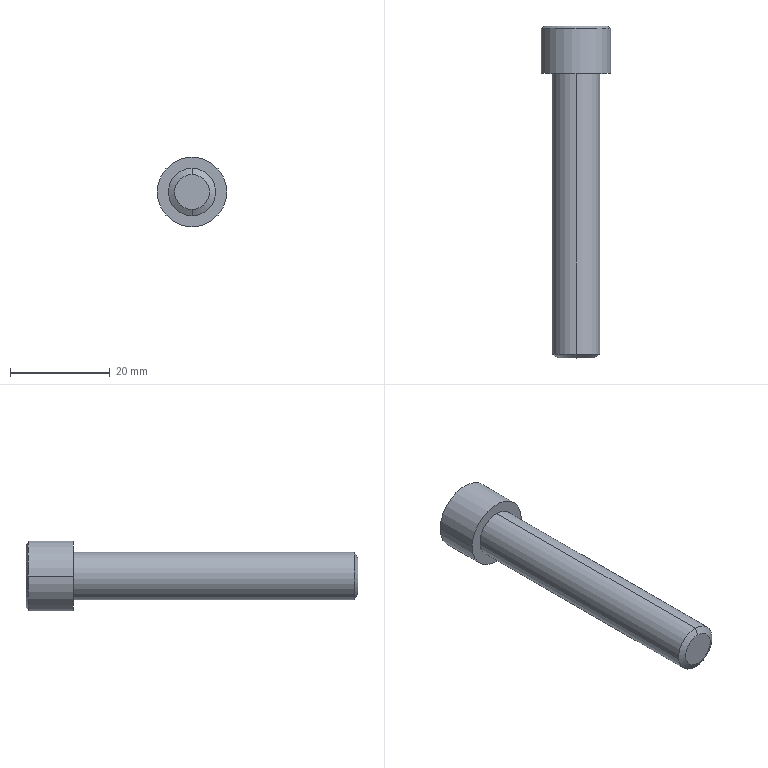Part | NX | features BREP 1 | 1 solid | 11 faces | box 13.97 x 66.675 x 13.97 mm | volume 5512 mm3 | cone 4 | cylinder 4 | plane 3 | commonest cylinder face diameters 9.525 x2 13.97 x2
STEP:
#1=CARTESIAN_POINT('',(0.,-57.15,3.493));
#2=VERTEX_POINT('',#1);
#3=CARTESIAN_POINT('',(0.,-57.15,-3.493));
#4=VERTEX_POINT('',#3);
#5=CARTESIAN_POINT('',(0.,-57.15,0.));
#6=DIRECTION('',(0.,-1.,0.));
#7=DIRECTION('',(0.,0.,1.));
#8=AXIS2_PLACEMENT_3D('',#5,#6,#7);
#9=CIRCLE('',#8,3.493);
#10=EDGE_CURVE('',#2,#4,#9,.T.);
#11=ORIENTED_EDGE('',*,*,#10,.T.);
#12=CARTESIAN_POINT('',(0.,-57.15,0.));
#13=DIRECTION('',(0.,-1.,0.));
#14=DIRECTION('',(0.,0.,-1.));
#15=AXIS2_PLACEMENT_3D('',#12,#13,#14);
#16=CIRCLE('',#15,3.493);
#17=EDGE_CURVE('',#4,#2,#16,.T.);
#18=ORIENTED_EDGE('',*,*,#17,.T.);
#19=EDGE_LOOP('',(#11,#18));
#20=FACE_BOUND('',#19,.T.);
#21=CARTESIAN_POINT('',(0.,-57.15,0.));
#22=DIRECTION('',(0.,-1.,0.));
#23=DIRECTION('',(0.,0.,-1.));
#24=AXIS2_PLACEMENT_3D('',#21,#22,#23);
#25=PLANE('',#24);
#26=ADVANCED_FACE('',(#20),#25,.T.);
#27=CARTESIAN_POINT('',(0.,-56.417,-4.763));
#28=VERTEX_POINT('',#27);
#29=CARTESIAN_POINT('',(0.,-57.15,-3.493));
#30=DIRECTION('',(0.,0.5,-0.866));
#31=VECTOR('',#30,1000.);
#32=LINE('',#29,#31);
#33=EDGE_CURVE('',#4,#28,#32,.T.);
#34=ORIENTED_EDGE('',*,*,#33,.T.);
#35=CARTESIAN_POINT('',(0.,-56.417,4.763));
#36=VERTEX_POINT('',#35);
#37=CARTESIAN_POINT('',(0.,-56.417,0.));
#38=DIRECTION('',(0.,-1.,0.));
#39=DIRECTION('',(0.,0.,-1.));
#40=AXIS2_PLACEMENT_3D('',#37,#38,#39);
#41=CIRCLE('',#40,4.763);
#42=EDGE_CURVE('',#28,#36,#41,.T.);
#43=ORIENTED_EDGE('',*,*,#42,.T.);
#44=CARTESIAN_POINT('',(0.,-57.15,3.493));
#45=DIRECTION('',(0.,0.5,0.866));
#46=VECTOR('',#45,1000.);
#47=LINE('',#44,#46);
#48=EDGE_CURVE('',#2,#36,#47,.T.);
#49=ORIENTED_EDGE('',*,*,#48,.F.);
#50=ORIENTED_EDGE('',*,*,#17,.F.);
#51=EDGE_LOOP('',(#34,#43,#49,#50));
#52=FACE_BOUND('',#51,.T.);
#53=CARTESIAN_POINT('',(0.,-56.783,0.));
#54=DIRECTION('',(0.,1.,0.));
#55=DIRECTION('',(0.,0.,1.));
#56=AXIS2_PLACEMENT_3D('',#53,#54,#55);
#57=CONICAL_SURFACE('',#56,4.128,1.047);
#58=ADVANCED_FACE('',(#52),#57,.T.);
#59=ORIENTED_EDGE('',*,*,#48,.T.);
#60=CARTESIAN_POINT('',(0.,-56.417,0.));
#61=DIRECTION('',(0.,-1.,0.));
#62=DIRECTION('',(0.,0.,1.));
#63=AXIS2_PLACEMENT_3D('',#60,#61,#62);
#64=CIRCLE('',#63,4.763);
#65=EDGE_CURVE('',#36,#28,#64,.T.);
#66=ORIENTED_EDGE('',*,*,#65,.T.);
#67=ORIENTED_EDGE('',*,*,#33,.F.);
#68=ORIENTED_EDGE('',*,*,#10,.F.);
#69=EDGE_LOOP('',(#59,#66,#67,#68));
#70=FACE_BOUND('',#69,.T.);
#71=CARTESIAN_POINT('',(0.,-56.783,0.));
#72=DIRECTION('',(0.,1.,0.));
#73=DIRECTION('',(0.,0.,1.));
#74=AXIS2_PLACEMENT_3D('',#71,#72,#73);
#75=CONICAL_SURFACE('',#74,4.128,1.047);
#76=ADVANCED_FACE('',(#70),#75,.T.);
#77=CARTESIAN_POINT('',(0.,0.,-4.763));
#78=VERTEX_POINT('',#77);
#79=CARTESIAN_POINT('',(0.,0.,-4.763));
#80=DIRECTION('',(0.,-1.,0.));
#81=VECTOR('',#80,1000.);
#82=LINE('',#79,#81);
#83=EDGE_CURVE('',#78,#28,#82,.T.);
#84=ORIENTED_EDGE('',*,*,#83,.T.);
#85=ORIENTED_EDGE('',*,*,#65,.F.);
#86=CARTESIAN_POINT('',(0.,0.,4.763));
#87=VERTEX_POINT('',#86);
#88=CARTESIAN_POINT('',(0.,0.,4.763));
#89=DIRECTION('',(0.,-1.,0.));
#90=VECTOR('',#89,1000.);
#91=LINE('',#88,#90);
#92=EDGE_CURVE('',#87,#36,#91,.T.);
#93=ORIENTED_EDGE('',*,*,#92,.F.);
#94=CARTESIAN_POINT('',(0.,0.,0.));
#95=DIRECTION('',(0.,-1.,0.));
#96=DIRECTION('',(0.,0.,1.));
#97=AXIS2_PLACEMENT_3D('',#94,#95,#96);
#98=CIRCLE('',#97,4.763);
#99=EDGE_CURVE('',#87,#78,#98,.T.);
#100=ORIENTED_EDGE('',*,*,#99,.T.);
#101=EDGE_LOOP('',(#84,#85,#93,#100));
#102=FACE_BOUND('',#101,.T.);
#103=CARTESIAN_POINT('',(0.,0.,0.));
#104=DIRECTION('',(0.,-1.,0.));
#105=DIRECTION('',(0.,0.,-1.));
#106=AXIS2_PLACEMENT_3D('',#103,#104,#105);
#107=CYLINDRICAL_SURFACE('',#106,4.763);
#108=ADVANCED_FACE('',(#102),#107,.T.);
#109=CARTESIAN_POINT('',(-6.985,0.,0.));
#110=VERTEX_POINT('',#109);
#111=CARTESIAN_POINT('',(6.985,0.,0.));
#112=VERTEX_POINT('',#111);
#113=CARTESIAN_POINT('',(0.,0.,0.));
#114=DIRECTION('',(0.,1.,0.));
#115=DIRECTION('',(-1.,0.,0.));
#116=AXIS2_PLACEMENT_3D('',#113,#114,#115);
#117=CIRCLE('',#116,6.985);
#118=EDGE_CURVE('',#110,#112,#117,.T.);
#119=ORIENTED_EDGE('',*,*,#118,.F.);
#120=CARTESIAN_POINT('',(0.,0.,0.));
#121=DIRECTION('',(0.,1.,0.));
#122=DIRECTION('',(1.,0.,0.));
#123=AXIS2_PLACEMENT_3D('',#120,#121,#122);
#124=CIRCLE('',#123,6.985);
#125=EDGE_CURVE('',#112,#110,#124,.T.);
#126=ORIENTED_EDGE('',*,*,#125,.F.);
#127=EDGE_LOOP('',(#119,#126));
#128=FACE_BOUND('',#127,.T.);
#129=ORIENTED_EDGE('',*,*,#99,.F.);
#130=CARTESIAN_POINT('',(0.,0.,0.));
#131=DIRECTION('',(0.,-1.,0.));
#132=DIRECTION('',(0.,0.,-1.));
#133=AXIS2_PLACEMENT_3D('',#130,#131,#132);
#134=CIRCLE('',#133,4.763);
#135=EDGE_CURVE('',#78,#87,#134,.T.);
#136=ORIENTED_EDGE('',*,*,#135,.F.);
#137=EDGE_LOOP('',(#129,#136));
#138=FACE_BOUND('',#137,.T.);
#139=CARTESIAN_POINT('',(0.,0.,0.));
#140=DIRECTION('',(0.,1.,0.));
#141=DIRECTION('',(1.,0.,0.));
#142=AXIS2_PLACEMENT_3D('',#139,#140,#141);
#143=PLANE('',#142);
#144=ADVANCED_FACE('',(#128,#138),#143,.F.);
#145=CARTESIAN_POINT('',(-6.985,9.085,0.));
#146=VERTEX_POINT('',#145);
#147=CARTESIAN_POINT('',(-6.985,0.,0.));
#148=DIRECTION('',(0.,1.,0.));
#149=VECTOR('',#148,1000.);
#150=LINE('',#147,#149);
#151=EDGE_CURVE('',#110,#146,#150,.T.);
#152=ORIENTED_EDGE('',*,*,#151,.T.);
#153=CARTESIAN_POINT('',(6.985,9.085,0.));
#154=VERTEX_POINT('',#153);
#155=CARTESIAN_POINT('',(0.,9.085,0.));
#156=DIRECTION('',(0.,1.,0.));
#157=DIRECTION('',(1.,0.,0.));
#158=AXIS2_PLACEMENT_3D('',#155,#156,#157);
#159=CIRCLE('',#158,6.985);
#160=EDGE_CURVE('',#154,#146,#159,.T.);
#161=ORIENTED_EDGE('',*,*,#160,.F.);
#162=CARTESIAN_POINT('',(6.985,0.,0.));
#163=DIRECTION('',(0.,1.,0.));
#164=VECTOR('',#163,1000.);
#165=LINE('',#162,#164);
#166=EDGE_CURVE('',#112,#154,#165,.T.);
#167=ORIENTED_EDGE('',*,*,#166,.F.);
#168=ORIENTED_EDGE('',*,*,#125,.T.);
#169=EDGE_LOOP('',(#152,#161,#167,#168));
#170=FACE_BOUND('',#169,.T.);
#171=CARTESIAN_POINT('',(0.,0.,0.));
#172=DIRECTION('',(0.,1.,0.));
#173=DIRECTION('',(1.,0.,0.));
#174=AXIS2_PLACEMENT_3D('',#171,#172,#173);
#175=CYLINDRICAL_SURFACE('',#174,6.985);
#176=ADVANCED_FACE('',(#170),#175,.T.);
#177=ORIENTED_EDGE('',*,*,#166,.T.);
#178=CARTESIAN_POINT('',(0.,9.085,0.));
#179=DIRECTION('',(0.,1.,0.));
#180=DIRECTION('',(-1.,0.,0.));
#181=AXIS2_PLACEMENT_3D('',#178,#179,#180);
#182=CIRCLE('',#181,6.985);
#183=EDGE_CURVE('',#146,#154,#182,.T.);
#184=ORIENTED_EDGE('',*,*,#183,.F.);
#185=ORIENTED_EDGE('',*,*,#151,.F.);
#186=ORIENTED_EDGE('',*,*,#118,.T.);
#187=EDGE_LOOP('',(#177,#184,#185,#186));
#188=FACE_BOUND('',#187,.T.);
#189=CARTESIAN_POINT('',(0.,0.,0.));
#190=DIRECTION('',(0.,1.,0.));
#191=DIRECTION('',(1.,0.,0.));
#192=AXIS2_PLACEMENT_3D('',#189,#190,#191);
#193=CYLINDRICAL_SURFACE('',#192,6.985);
#194=ADVANCED_FACE('',(#188),#193,.T.);
#195=CARTESIAN_POINT('',(-6.223,9.525,0.));
#196=VERTEX_POINT('',#195);
#197=CARTESIAN_POINT('',(-6.223,9.525,0.));
#198=DIRECTION('',(-0.866,-0.5,0.));
#199=VECTOR('',#198,1000.);
#200=LINE('',#197,#199);
#201=EDGE_CURVE('',#196,#146,#200,.T.);
#202=ORIENTED_EDGE('',*,*,#201,.T.);
#203=ORIENTED_EDGE('',*,*,#183,.T.);
#204=CARTESIAN_POINT('',(6.223,9.525,0.));
#205=VERTEX_POINT('',#204);
#206=CARTESIAN_POINT('',(6.223,9.525,0.));
#207=DIRECTION('',(0.866,-0.5,0.));
#208=VECTOR('',#207,1000.);
#209=LINE('',#206,#208);
#210=EDGE_CURVE('',#205,#154,#209,.T.);
#211=ORIENTED_EDGE('',*,*,#210,.F.);
#212=CARTESIAN_POINT('',(0.,9.525,0.));
#213=DIRECTION('',(0.,1.,0.));
#214=DIRECTION('',(-1.,0.,0.));
#215=AXIS2_PLACEMENT_3D('',#212,#213,#214);
#216=CIRCLE('',#215,6.223);
#217=EDGE_CURVE('',#196,#205,#216,.T.);
#218=ORIENTED_EDGE('',*,*,#217,.F.);
#219=EDGE_LOOP('',(#202,#203,#211,#218));
#220=FACE_BOUND('',#219,.T.);
#221=CARTESIAN_POINT('',(0.,9.305,0.));
#222=DIRECTION('',(0.,-1.,0.));
#223=DIRECTION('',(-1.,0.,0.));
#224=AXIS2_PLACEMENT_3D('',#221,#222,#223);
#225=CONICAL_SURFACE('',#224,6.604,1.047);
#226=ADVANCED_FACE('',(#220),#225,.T.);
#227=ORIENTED_EDGE('',*,*,#217,.T.);
#228=CARTESIAN_POINT('',(0.,9.525,0.));
#229=DIRECTION('',(0.,1.,0.));
#230=DIRECTION('',(1.,0.,0.));
#231=AXIS2_PLACEMENT_3D('',#228,#229,#230);
#232=CIRCLE('',#231,6.223);
#233=EDGE_CURVE('',#205,#196,#232,.T.);
#234=ORIENTED_EDGE('',*,*,#233,.T.);
#235=EDGE_LOOP('',(#227,#234));
#236=FACE_BOUND('',#235,.T.);
#237=CARTESIAN_POINT('',(0.,9.525,0.));
#238=DIRECTION('',(0.,1.,0.));
#239=DIRECTION('',(1.,0.,0.));
#240=AXIS2_PLACEMENT_3D('',#237,#238,#239);
#241=PLANE('',#240);
#242=ADVANCED_FACE('',(#236),#241,.T.);
#243=ORIENTED_EDGE('',*,*,#210,.T.);
#244=ORIENTED_EDGE('',*,*,#160,.T.);
#245=ORIENTED_EDGE('',*,*,#201,.F.);
#246=ORIENTED_EDGE('',*,*,#233,.F.);
#247=EDGE_LOOP('',(#243,#244,#245,#246));
#248=FACE_BOUND('',#247,.T.);
#249=CARTESIAN_POINT('',(0.,9.305,0.));
#250=DIRECTION('',(0.,-1.,0.));
#251=DIRECTION('',(-1.,0.,0.));
#252=AXIS2_PLACEMENT_3D('',#249,#250,#251);
#253=CONICAL_SURFACE('',#252,6.604,1.047);
#254=ADVANCED_FACE('',(#248),#253,.T.);
#255=ORIENTED_EDGE('',*,*,#92,.T.);
#256=ORIENTED_EDGE('',*,*,#42,.F.);
#257=ORIENTED_EDGE('',*,*,#83,.F.);
#258=ORIENTED_EDGE('',*,*,#135,.T.);
#259=EDGE_LOOP('',(#255,#256,#257,#258));
#260=FACE_BOUND('',#259,.T.);
#261=CARTESIAN_POINT('',(0.,0.,0.));
#262=DIRECTION('',(0.,-1.,0.));
#263=DIRECTION('',(0.,0.,-1.));
#264=AXIS2_PLACEMENT_3D('',#261,#262,#263);
#265=CYLINDRICAL_SURFACE('',#264,4.763);
#266=ADVANCED_FACE('',(#260),#265,.T.);
#267=CLOSED_SHELL('',(#26,#58,#76,#108,#144,#176,#194,#226,#242,#254,#266));
#268=MANIFOLD_SOLID_BREP('',#267);
#269=(LENGTH_UNIT()NAMED_UNIT(*)SI_UNIT(.MILLI.,.METRE.));
#270=UNCERTAINTY_MEASURE_WITH_UNIT(LENGTH_MEASURE(0.00001),#269,'','');
#271=(NAMED_UNIT(*)PLANE_ANGLE_UNIT()SI_UNIT($,.RADIAN.));
#272=(NAMED_UNIT(*)SI_UNIT($,.STERADIAN.)SOLID_ANGLE_UNIT());
#273=(GEOMETRIC_REPRESENTATION_CONTEXT(3)GLOBAL_UNCERTAINTY_ASSIGNED_CONTEXT((#270))GLOBAL_UNIT_ASSIGNED_CONTEXT((#269,#271,#272))REPRESENTATION_CONTEXT('',''));
#274=ADVANCED_BREP_SHAPE_REPRESENTATION('',(#268),#273);